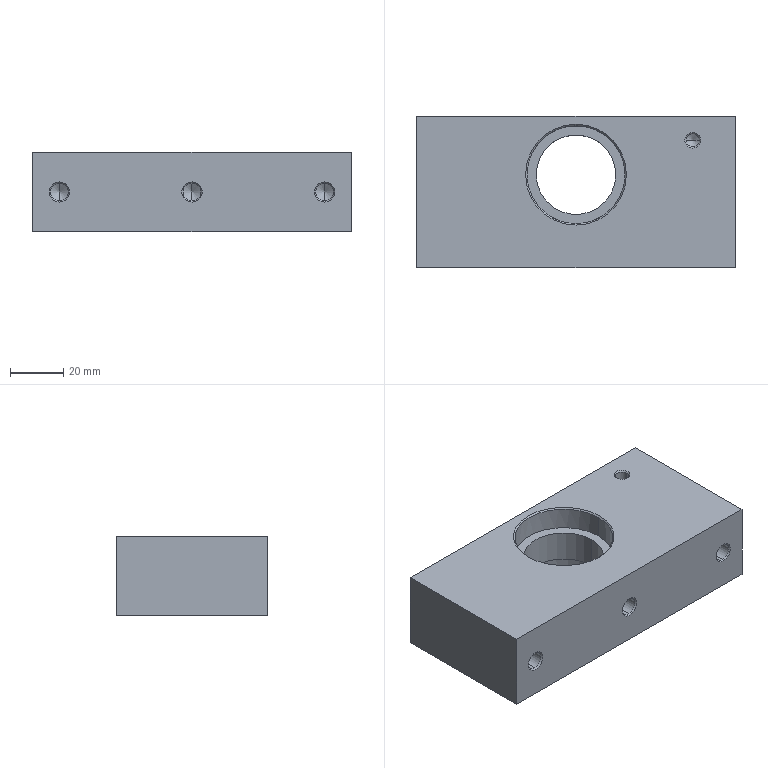Part | STEP file | Roller base | 1 solid | 54 faces | box 120 x 57 x 30 mm | volume 174440 mm3 | cone 28 | cylinder 18 | plane 8 | commonest cylinder face diameters 6.647 x10 37 x4 4.917 x2 30 x2